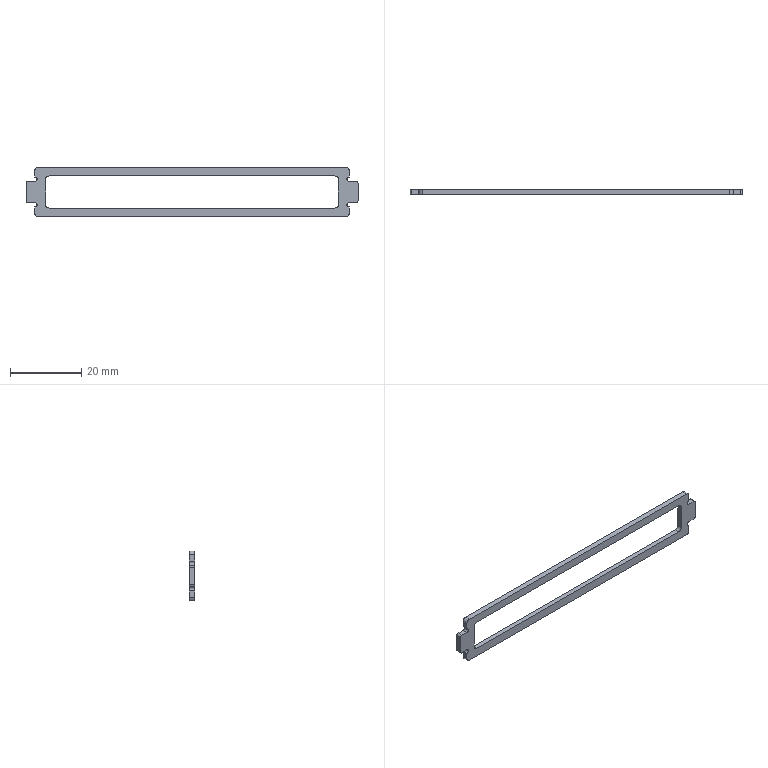Part | SolidWorks | features Fillet 2, Extrusion 1 | 1 solid | 34 faces | box 93.2 x 1.5 x 14 mm | volume 783.785 mm3 | plane 18 | cylinder 16 | commonest cylinder face diameters 2 x8 1 x4 1.2 x4
STEP:
#1=CARTESIAN_POINT('',(-44.1,1.5,-6.));
#2=VERTEX_POINT('',#1);
#3=CARTESIAN_POINT('',(-44.1,1.5,-4.2));
#4=VERTEX_POINT('',#3);
#5=CARTESIAN_POINT('',(-44.1,1.5,0.));
#6=DIRECTION('',(0.,0.,1.));
#7=VECTOR('',#6,1000.);
#8=LINE('',#5,#7);
#9=EDGE_CURVE('',#2,#4,#8,.T.);
#10=ORIENTED_EDGE('',*,*,#9,.F.);
#11=CARTESIAN_POINT('',(-44.1,0.,-6.));
#12=VERTEX_POINT('',#11);
#13=CARTESIAN_POINT('',(-44.1,0.,-6.));
#14=DIRECTION('',(0.,-1.,0.));
#15=VECTOR('',#14,1000.);
#16=LINE('',#13,#15);
#17=EDGE_CURVE('',#2,#12,#16,.T.);
#18=ORIENTED_EDGE('',*,*,#17,.T.);
#19=CARTESIAN_POINT('',(-44.1,0.,-4.2));
#20=VERTEX_POINT('',#19);
#21=CARTESIAN_POINT('',(-44.1,0.,0.));
#22=DIRECTION('',(0.,0.,1.));
#23=VECTOR('',#22,1000.);
#24=LINE('',#21,#23);
#25=EDGE_CURVE('',#12,#20,#24,.T.);
#26=ORIENTED_EDGE('',*,*,#25,.T.);
#27=CARTESIAN_POINT('',(-44.1,1.5,-4.2));
#28=DIRECTION('',(0.,-1.,0.));
#29=VECTOR('',#28,1000.);
#30=LINE('',#27,#29);
#31=EDGE_CURVE('',#4,#20,#30,.T.);
#32=ORIENTED_EDGE('',*,*,#31,.F.);
#33=EDGE_LOOP('',(#10,#18,#26,#32));
#34=FACE_OUTER_BOUND('',#33,.T.);
#35=CARTESIAN_POINT('',(-44.1,1.5,0.));
#36=DIRECTION('',(1.,0.,0.));
#37=DIRECTION('',(0.,0.,-1.));
#38=AXIS2_PLACEMENT_3D('',#35,#36,#37);
#39=PLANE('',#38);
#40=ADVANCED_FACE('',(#34),#39,.F.);
#41=CARTESIAN_POINT('',(-44.1,0.,-3.));
#42=VERTEX_POINT('',#41);
#43=CARTESIAN_POINT('',(-44.1,0.,-3.6));
#44=DIRECTION('',(0.,-1.,0.));
#45=DIRECTION('',(0.,0.,1.));
#46=AXIS2_PLACEMENT_3D('',#43,#44,#45);
#47=CIRCLE('',#46,0.6);
#48=EDGE_CURVE('',#20,#42,#47,.T.);
#49=ORIENTED_EDGE('',*,*,#48,.T.);
#50=CARTESIAN_POINT('',(-44.1,1.5,-3.));
#51=VERTEX_POINT('',#50);
#52=CARTESIAN_POINT('',(-44.1,1.5,-3.));
#53=DIRECTION('',(0.,-1.,0.));
#54=VECTOR('',#53,1000.);
#55=LINE('',#52,#54);
#56=EDGE_CURVE('',#51,#42,#55,.T.);
#57=ORIENTED_EDGE('',*,*,#56,.F.);
#58=CARTESIAN_POINT('',(-44.1,1.5,-3.6));
#59=DIRECTION('',(0.,-1.,0.));
#60=DIRECTION('',(0.,0.,1.));
#61=AXIS2_PLACEMENT_3D('',#58,#59,#60);
#62=CIRCLE('',#61,0.6);
#63=EDGE_CURVE('',#4,#51,#62,.T.);
#64=ORIENTED_EDGE('',*,*,#63,.F.);
#65=ORIENTED_EDGE('',*,*,#31,.T.);
#66=EDGE_LOOP('',(#49,#57,#64,#65));
#67=FACE_OUTER_BOUND('',#66,.T.);
#68=CARTESIAN_POINT('',(-44.1,1.5,-3.6));
#69=DIRECTION('',(0.,-1.,0.));
#70=DIRECTION('',(0.,0.,-1.));
#71=AXIS2_PLACEMENT_3D('',#68,#69,#70);
#72=CYLINDRICAL_SURFACE('',#71,0.6);
#73=ADVANCED_FACE('',(#67),#72,.F.);
#74=CARTESIAN_POINT('',(-46.1,0.,-3.));
#75=VERTEX_POINT('',#74);
#76=CARTESIAN_POINT('',(0.,0.,-3.));
#77=DIRECTION('',(-1.,0.,0.));
#78=VECTOR('',#77,1000.);
#79=LINE('',#76,#78);
#80=EDGE_CURVE('',#42,#75,#79,.T.);
#81=ORIENTED_EDGE('',*,*,#80,.T.);
#82=CARTESIAN_POINT('',(-46.1,1.5,-3.));
#83=VERTEX_POINT('',#82);
#84=CARTESIAN_POINT('',(-46.1,1.5,-3.));
#85=DIRECTION('',(0.,1.,0.));
#86=VECTOR('',#85,1000.);
#87=LINE('',#84,#86);
#88=EDGE_CURVE('',#75,#83,#87,.T.);
#89=ORIENTED_EDGE('',*,*,#88,.T.);
#90=CARTESIAN_POINT('',(0.,1.5,-3.));
#91=DIRECTION('',(-1.,0.,0.));
#92=VECTOR('',#91,1000.);
#93=LINE('',#90,#92);
#94=EDGE_CURVE('',#51,#83,#93,.T.);
#95=ORIENTED_EDGE('',*,*,#94,.F.);
#96=ORIENTED_EDGE('',*,*,#56,.T.);
#97=EDGE_LOOP('',(#81,#89,#95,#96));
#98=FACE_OUTER_BOUND('',#97,.T.);
#99=CARTESIAN_POINT('',(0.,1.5,-3.));
#100=DIRECTION('',(0.,0.,1.));
#101=DIRECTION('',(1.,0.,0.));
#102=AXIS2_PLACEMENT_3D('',#99,#100,#101);
#103=PLANE('',#102);
#104=ADVANCED_FACE('',(#98),#103,.F.);
#105=CARTESIAN_POINT('',(-46.6,0.,-2.5));
#106=VERTEX_POINT('',#105);
#107=CARTESIAN_POINT('',(-46.6,0.,2.5));
#108=VERTEX_POINT('',#107);
#109=CARTESIAN_POINT('',(-46.6,0.,0.));
#110=DIRECTION('',(0.,0.,1.));
#111=VECTOR('',#110,1000.);
#112=LINE('',#109,#111);
#113=EDGE_CURVE('',#106,#108,#112,.T.);
#114=ORIENTED_EDGE('',*,*,#113,.T.);
#115=CARTESIAN_POINT('',(-46.6,1.5,2.5));
#116=VERTEX_POINT('',#115);
#117=CARTESIAN_POINT('',(-46.6,1.5,2.5));
#118=DIRECTION('',(0.,1.,0.));
#119=VECTOR('',#118,1000.);
#120=LINE('',#117,#119);
#121=EDGE_CURVE('',#108,#116,#120,.T.);
#122=ORIENTED_EDGE('',*,*,#121,.T.);
#123=CARTESIAN_POINT('',(-46.6,1.5,-2.5));
#124=VERTEX_POINT('',#123);
#125=CARTESIAN_POINT('',(-46.6,1.5,0.));
#126=DIRECTION('',(0.,0.,1.));
#127=VECTOR('',#126,1000.);
#128=LINE('',#125,#127);
#129=EDGE_CURVE('',#124,#116,#128,.T.);
#130=ORIENTED_EDGE('',*,*,#129,.F.);
#131=CARTESIAN_POINT('',(-46.6,1.5,-2.5));
#132=DIRECTION('',(0.,-1.,0.));
#133=VECTOR('',#132,1000.);
#134=LINE('',#131,#133);
#135=EDGE_CURVE('',#124,#106,#134,.T.);
#136=ORIENTED_EDGE('',*,*,#135,.T.);
#137=EDGE_LOOP('',(#114,#122,#130,#136));
#138=FACE_OUTER_BOUND('',#137,.T.);
#139=CARTESIAN_POINT('',(-46.6,1.5,0.));
#140=DIRECTION('',(1.,0.,0.));
#141=DIRECTION('',(0.,0.,-1.));
#142=AXIS2_PLACEMENT_3D('',#139,#140,#141);
#143=PLANE('',#142);
#144=ADVANCED_FACE('',(#138),#143,.F.);
#145=CARTESIAN_POINT('',(-44.1,1.5,3.));
#146=VERTEX_POINT('',#145);
#147=CARTESIAN_POINT('',(-46.1,1.5,3.));
#148=VERTEX_POINT('',#147);
#149=CARTESIAN_POINT('',(0.,1.5,3.));
#150=DIRECTION('',(-1.,0.,0.));
#151=VECTOR('',#150,1000.);
#152=LINE('',#149,#151);
#153=EDGE_CURVE('',#146,#148,#152,.T.);
#154=ORIENTED_EDGE('',*,*,#153,.T.);
#155=CARTESIAN_POINT('',(-46.1,0.,3.));
#156=VERTEX_POINT('',#155);
#157=CARTESIAN_POINT('',(-46.1,0.,3.));
#158=DIRECTION('',(0.,-1.,0.));
#159=VECTOR('',#158,1000.);
#160=LINE('',#157,#159);
#161=EDGE_CURVE('',#148,#156,#160,.T.);
#162=ORIENTED_EDGE('',*,*,#161,.T.);
#163=CARTESIAN_POINT('',(-44.1,0.,3.));
#164=VERTEX_POINT('',#163);
#165=CARTESIAN_POINT('',(0.,0.,3.));
#166=DIRECTION('',(-1.,0.,0.));
#167=VECTOR('',#166,1000.);
#168=LINE('',#165,#167);
#169=EDGE_CURVE('',#164,#156,#168,.T.);
#170=ORIENTED_EDGE('',*,*,#169,.F.);
#171=CARTESIAN_POINT('',(-44.1,1.5,3.));
#172=DIRECTION('',(0.,-1.,0.));
#173=VECTOR('',#172,1000.);
#174=LINE('',#171,#173);
#175=EDGE_CURVE('',#146,#164,#174,.T.);
#176=ORIENTED_EDGE('',*,*,#175,.F.);
#177=EDGE_LOOP('',(#154,#162,#170,#176));
#178=FACE_OUTER_BOUND('',#177,.T.);
#179=CARTESIAN_POINT('',(0.,1.5,3.));
#180=DIRECTION('',(0.,0.,1.));
#181=DIRECTION('',(1.,0.,0.));
#182=AXIS2_PLACEMENT_3D('',#179,#180,#181);
#183=PLANE('',#182);
#184=ADVANCED_FACE('',(#178),#183,.T.);
#185=CARTESIAN_POINT('',(-44.1,0.,4.2));
#186=VERTEX_POINT('',#185);
#187=CARTESIAN_POINT('',(-44.1,0.,3.6));
#188=DIRECTION('',(0.,-1.,0.));
#189=DIRECTION('',(0.,0.,1.));
#190=AXIS2_PLACEMENT_3D('',#187,#188,#189);
#191=CIRCLE('',#190,0.6);
#192=EDGE_CURVE('',#164,#186,#191,.T.);
#193=ORIENTED_EDGE('',*,*,#192,.T.);
#194=CARTESIAN_POINT('',(-44.1,1.5,4.2));
#195=VERTEX_POINT('',#194);
#196=CARTESIAN_POINT('',(-44.1,1.5,4.2));
#197=DIRECTION('',(0.,-1.,0.));
#198=VECTOR('',#197,1000.);
#199=LINE('',#196,#198);
#200=EDGE_CURVE('',#195,#186,#199,.T.);
#201=ORIENTED_EDGE('',*,*,#200,.F.);
#202=CARTESIAN_POINT('',(-44.1,1.5,3.6));
#203=DIRECTION('',(0.,-1.,0.));
#204=DIRECTION('',(0.,0.,1.));
#205=AXIS2_PLACEMENT_3D('',#202,#203,#204);
#206=CIRCLE('',#205,0.6);
#207=EDGE_CURVE('',#146,#195,#206,.T.);
#208=ORIENTED_EDGE('',*,*,#207,.F.);
#209=ORIENTED_EDGE('',*,*,#175,.T.);
#210=EDGE_LOOP('',(#193,#201,#208,#209));
#211=FACE_OUTER_BOUND('',#210,.T.);
#212=CARTESIAN_POINT('',(-44.1,1.5,3.6));
#213=DIRECTION('',(0.,-1.,0.));
#214=DIRECTION('',(0.,0.,-1.));
#215=AXIS2_PLACEMENT_3D('',#212,#213,#214);
#216=CYLINDRICAL_SURFACE('',#215,0.6);
#217=ADVANCED_FACE('',(#211),#216,.F.);
#218=CARTESIAN_POINT('',(-44.1,0.,6.));
#219=VERTEX_POINT('',#218);
#220=CARTESIAN_POINT('',(-44.1,0.,0.));
#221=DIRECTION('',(0.,0.,1.));
#222=VECTOR('',#221,1000.);
#223=LINE('',#220,#222);
#224=EDGE_CURVE('',#186,#219,#223,.T.);
#225=ORIENTED_EDGE('',*,*,#224,.T.);
#226=CARTESIAN_POINT('',(-44.1,1.5,6.));
#227=VERTEX_POINT('',#226);
#228=CARTESIAN_POINT('',(-44.1,1.5,6.));
#229=DIRECTION('',(0.,1.,0.));
#230=VECTOR('',#229,1000.);
#231=LINE('',#228,#230);
#232=EDGE_CURVE('',#219,#227,#231,.T.);
#233=ORIENTED_EDGE('',*,*,#232,.T.);
#234=CARTESIAN_POINT('',(-44.1,1.5,0.));
#235=DIRECTION('',(0.,0.,1.));
#236=VECTOR('',#235,1000.);
#237=LINE('',#234,#236);
#238=EDGE_CURVE('',#195,#227,#237,.T.);
#239=ORIENTED_EDGE('',*,*,#238,.F.);
#240=ORIENTED_EDGE('',*,*,#200,.T.);
#241=EDGE_LOOP('',(#225,#233,#239,#240));
#242=FACE_OUTER_BOUND('',#241,.T.);
#243=CARTESIAN_POINT('',(-44.1,1.5,0.));
#244=DIRECTION('',(1.,0.,0.));
#245=DIRECTION('',(0.,0.,-1.));
#246=AXIS2_PLACEMENT_3D('',#243,#244,#245);
#247=PLANE('',#246);
#248=ADVANCED_FACE('',(#242),#247,.F.);
#249=CARTESIAN_POINT('',(-43.1,1.5,7.));
#250=VERTEX_POINT('',#249);
#251=CARTESIAN_POINT('',(43.1,1.5,7.));
#252=VERTEX_POINT('',#251);
#253=CARTESIAN_POINT('',(0.,1.5,7.));
#254=DIRECTION('',(1.,0.,0.));
#255=VECTOR('',#254,1000.);
#256=LINE('',#253,#255);
#257=EDGE_CURVE('',#250,#252,#256,.T.);
#258=ORIENTED_EDGE('',*,*,#257,.F.);
#259=CARTESIAN_POINT('',(-43.1,0.,7.));
#260=VERTEX_POINT('',#259);
#261=CARTESIAN_POINT('',(-43.1,1.5,7.));
#262=DIRECTION('',(0.,-1.,0.));
#263=VECTOR('',#262,1000.);
#264=LINE('',#261,#263);
#265=EDGE_CURVE('',#250,#260,#264,.T.);
#266=ORIENTED_EDGE('',*,*,#265,.T.);
#267=CARTESIAN_POINT('',(43.1,0.,7.));
#268=VERTEX_POINT('',#267);
#269=CARTESIAN_POINT('',(0.,0.,7.));
#270=DIRECTION('',(1.,0.,0.));
#271=VECTOR('',#270,1000.);
#272=LINE('',#269,#271);
#273=EDGE_CURVE('',#260,#268,#272,.T.);
#274=ORIENTED_EDGE('',*,*,#273,.T.);
#275=CARTESIAN_POINT('',(43.1,1.5,7.));
#276=DIRECTION('',(0.,1.,0.));
#277=VECTOR('',#276,1000.);
#278=LINE('',#275,#277);
#279=EDGE_CURVE('',#268,#252,#278,.T.);
#280=ORIENTED_EDGE('',*,*,#279,.T.);
#281=EDGE_LOOP('',(#258,#266,#274,#280));
#282=FACE_OUTER_BOUND('',#281,.T.);
#283=CARTESIAN_POINT('',(0.,1.5,7.));
#284=DIRECTION('',(0.,0.,-1.));
#285=DIRECTION('',(-1.,0.,0.));
#286=AXIS2_PLACEMENT_3D('',#283,#284,#285);
#287=PLANE('',#286);
#288=ADVANCED_FACE('',(#282),#287,.F.);
#289=CARTESIAN_POINT('',(44.1,1.5,4.2));
#290=VERTEX_POINT('',#289);
#291=CARTESIAN_POINT('',(44.1,1.5,6.));
#292=VERTEX_POINT('',#291);
#293=CARTESIAN_POINT('',(44.1,1.5,0.));
#294=DIRECTION('',(0.,0.,1.));
#295=VECTOR('',#294,1000.);
#296=LINE('',#293,#295);
#297=EDGE_CURVE('',#290,#292,#296,.T.);
#298=ORIENTED_EDGE('',*,*,#297,.T.);
#299=CARTESIAN_POINT('',(44.1,0.,6.));
#300=VERTEX_POINT('',#299);
#301=CARTESIAN_POINT('',(44.1,0.,6.));
#302=DIRECTION('',(0.,-1.,0.));
#303=VECTOR('',#302,1000.);
#304=LINE('',#301,#303);
#305=EDGE_CURVE('',#292,#300,#304,.T.);
#306=ORIENTED_EDGE('',*,*,#305,.T.);
#307=CARTESIAN_POINT('',(44.1,0.,4.2));
#308=VERTEX_POINT('',#307);
#309=CARTESIAN_POINT('',(44.1,0.,0.));
#310=DIRECTION('',(0.,0.,1.));
#311=VECTOR('',#310,1000.);
#312=LINE('',#309,#311);
#313=EDGE_CURVE('',#308,#300,#312,.T.);
#314=ORIENTED_EDGE('',*,*,#313,.F.);
#315=CARTESIAN_POINT('',(44.1,1.5,4.2));
#316=DIRECTION('',(0.,-1.,0.));
#317=VECTOR('',#316,1000.);
#318=LINE('',#315,#317);
#319=EDGE_CURVE('',#290,#308,#318,.T.);
#320=ORIENTED_EDGE('',*,*,#319,.F.);
#321=EDGE_LOOP('',(#298,#306,#314,#320));
#322=FACE_OUTER_BOUND('',#321,.T.);
#323=CARTESIAN_POINT('',(44.1,1.5,0.));
#324=DIRECTION('',(1.,0.,0.));
#325=DIRECTION('',(0.,0.,-1.));
#326=AXIS2_PLACEMENT_3D('',#323,#324,#325);
#327=PLANE('',#326);
#328=ADVANCED_FACE('',(#322),#327,.T.);
#329=CARTESIAN_POINT('',(44.1,0.,3.));
#330=VERTEX_POINT('',#329);
#331=CARTESIAN_POINT('',(44.1,0.,3.6));
#332=DIRECTION('',(0.,1.,0.));
#333=DIRECTION('',(0.,0.,1.));
#334=AXIS2_PLACEMENT_3D('',#331,#332,#333);
#335=CIRCLE('',#334,0.6);
#336=EDGE_CURVE('',#330,#308,#335,.T.);
#337=ORIENTED_EDGE('',*,*,#336,.F.);
#338=CARTESIAN_POINT('',(44.1,1.5,3.));
#339=VERTEX_POINT('',#338);
#340=CARTESIAN_POINT('',(44.1,1.5,3.));
#341=DIRECTION('',(0.,-1.,0.));
#342=VECTOR('',#341,1000.);
#343=LINE('',#340,#342);
#344=EDGE_CURVE('',#339,#330,#343,.T.);
#345=ORIENTED_EDGE('',*,*,#344,.F.);
#346=CARTESIAN_POINT('',(44.1,1.5,3.6));
#347=DIRECTION('',(0.,1.,0.));
#348=DIRECTION('',(0.,0.,1.));
#349=AXIS2_PLACEMENT_3D('',#346,#347,#348);
#350=CIRCLE('',#349,0.6);
#351=EDGE_CURVE('',#339,#290,#350,.T.);
#352=ORIENTED_EDGE('',*,*,#351,.T.);
#353=ORIENTED_EDGE('',*,*,#319,.T.);
#354=EDGE_LOOP('',(#337,#345,#352,#353));
#355=FACE_OUTER_BOUND('',#354,.T.);
#356=CARTESIAN_POINT('',(44.1,1.5,3.6));
#357=DIRECTION('',(0.,-1.,0.));
#358=DIRECTION('',(0.,0.,-1.));
#359=AXIS2_PLACEMENT_3D('',#356,#357,#358);
#360=CYLINDRICAL_SURFACE('',#359,0.6);
#361=ADVANCED_FACE('',(#355),#360,.F.);
#362=CARTESIAN_POINT('',(46.1,0.,3.));
#363=VERTEX_POINT('',#362);
#364=CARTESIAN_POINT('',(0.,0.,3.));
#365=DIRECTION('',(1.,0.,0.));
#366=VECTOR('',#365,1000.);
#367=LINE('',#364,#366);
#368=EDGE_CURVE('',#330,#363,#367,.T.);
#369=ORIENTED_EDGE('',*,*,#368,.T.);
#370=CARTESIAN_POINT('',(46.1,1.5,3.));
#371=VERTEX_POINT('',#370);
#372=CARTESIAN_POINT('',(46.1,1.5,3.));
#373=DIRECTION('',(0.,1.,0.));
#374=VECTOR('',#373,1000.);
#375=LINE('',#372,#374);
#376=EDGE_CURVE('',#363,#371,#375,.T.);
#377=ORIENTED_EDGE('',*,*,#376,.T.);
#378=CARTESIAN_POINT('',(0.,1.5,3.));
#379=DIRECTION('',(1.,0.,0.));
#380=VECTOR('',#379,1000.);
#381=LINE('',#378,#380);
#382=EDGE_CURVE('',#339,#371,#381,.T.);
#383=ORIENTED_EDGE('',*,*,#382,.F.);
#384=ORIENTED_EDGE('',*,*,#344,.T.);
#385=EDGE_LOOP('',(#369,#377,#383,#384));
#386=FACE_OUTER_BOUND('',#385,.T.);
#387=CARTESIAN_POINT('',(0.,1.5,3.));
#388=DIRECTION('',(0.,0.,-1.));
#389=DIRECTION('',(-1.,0.,0.));
#390=AXIS2_PLACEMENT_3D('',#387,#388,#389);
#391=PLANE('',#390);
#392=ADVANCED_FACE('',(#386),#391,.F.);
#393=CARTESIAN_POINT('',(46.6,1.5,-2.5));
#394=VERTEX_POINT('',#393);
#395=CARTESIAN_POINT('',(46.6,1.5,2.5));
#396=VERTEX_POINT('',#395);
#397=CARTESIAN_POINT('',(46.6,1.5,0.));
#398=DIRECTION('',(0.,0.,1.));
#399=VECTOR('',#398,1000.);
#400=LINE('',#397,#399);
#401=EDGE_CURVE('',#394,#396,#400,.T.);
#402=ORIENTED_EDGE('',*,*,#401,.T.);
#403=CARTESIAN_POINT('',(46.6,0.,2.5));
#404=VERTEX_POINT('',#403);
#405=CARTESIAN_POINT('',(46.6,0.,2.5));
#406=DIRECTION('',(0.,-1.,0.));
#407=VECTOR('',#406,1000.);
#408=LINE('',#405,#407);
#409=EDGE_CURVE('',#396,#404,#408,.T.);
#410=ORIENTED_EDGE('',*,*,#409,.T.);
#411=CARTESIAN_POINT('',(46.6,0.,-2.5));
#412=VERTEX_POINT('',#411);
#413=CARTESIAN_POINT('',(46.6,0.,0.));
#414=DIRECTION('',(0.,0.,1.));
#415=VECTOR('',#414,1000.);
#416=LINE('',#413,#415);
#417=EDGE_CURVE('',#412,#404,#416,.T.);
#418=ORIENTED_EDGE('',*,*,#417,.F.);
#419=CARTESIAN_POINT('',(46.6,1.5,-2.5));
#420=DIRECTION('',(0.,1.,0.));
#421=VECTOR('',#420,1000.);
#422=LINE('',#419,#421);
#423=EDGE_CURVE('',#412,#394,#422,.T.);
#424=ORIENTED_EDGE('',*,*,#423,.T.);
#425=EDGE_LOOP('',(#402,#410,#418,#424));
#426=FACE_OUTER_BOUND('',#425,.T.);
#427=CARTESIAN_POINT('',(46.6,1.5,0.));
#428=DIRECTION('',(1.,0.,0.));
#429=DIRECTION('',(0.,0.,-1.));
#430=AXIS2_PLACEMENT_3D('',#427,#428,#429);
#431=PLANE('',#430);
#432=ADVANCED_FACE('',(#426),#431,.T.);
#433=CARTESIAN_POINT('',(44.1,1.5,-3.));
#434=VERTEX_POINT('',#433);
#435=CARTESIAN_POINT('',(46.1,1.5,-3.));
#436=VERTEX_POINT('',#435);
#437=CARTESIAN_POINT('',(0.,1.5,-3.));
#438=DIRECTION('',(1.,0.,0.));
#439=VECTOR('',#438,1000.);
#440=LINE('',#437,#439);
#441=EDGE_CURVE('',#434,#436,#440,.T.);
#442=ORIENTED_EDGE('',*,*,#441,.T.);
#443=CARTESIAN_POINT('',(46.1,0.,-3.));
#444=VERTEX_POINT('',#443);
#445=CARTESIAN_POINT('',(46.1,1.5,-3.));
#446=DIRECTION('',(0.,-1.,0.));
#447=VECTOR('',#446,1000.);
#448=LINE('',#445,#447);
#449=EDGE_CURVE('',#436,#444,#448,.T.);
#450=ORIENTED_EDGE('',*,*,#449,.T.);
#451=CARTESIAN_POINT('',(44.1,0.,-3.));
#452=VERTEX_POINT('',#451);
#453=CARTESIAN_POINT('',(0.,0.,-3.));
#454=DIRECTION('',(1.,0.,0.));
#455=VECTOR('',#454,1000.);
#456=LINE('',#453,#455);
#457=EDGE_CURVE('',#452,#444,#456,.T.);
#458=ORIENTED_EDGE('',*,*,#457,.F.);
#459=CARTESIAN_POINT('',(44.1,1.5,-3.));
#460=DIRECTION('',(0.,-1.,0.));
#461=VECTOR('',#460,1000.);
#462=LINE('',#459,#461);
#463=EDGE_CURVE('',#434,#452,#462,.T.);
#464=ORIENTED_EDGE('',*,*,#463,.F.);
#465=EDGE_LOOP('',(#442,#450,#458,#464));
#466=FACE_OUTER_BOUND('',#465,.T.);
#467=CARTESIAN_POINT('',(0.,1.5,-3.));
#468=DIRECTION('',(0.,0.,-1.));
#469=DIRECTION('',(-1.,0.,0.));
#470=AXIS2_PLACEMENT_3D('',#467,#468,#469);
#471=PLANE('',#470);
#472=ADVANCED_FACE('',(#466),#471,.T.);
#473=CARTESIAN_POINT('',(44.1,0.,-4.2));
#474=VERTEX_POINT('',#473);
#475=CARTESIAN_POINT('',(44.1,0.,-3.6));
#476=DIRECTION('',(0.,1.,0.));
#477=DIRECTION('',(0.,0.,1.));
#478=AXIS2_PLACEMENT_3D('',#475,#476,#477);
#479=CIRCLE('',#478,0.6);
#480=EDGE_CURVE('',#474,#452,#479,.T.);
#481=ORIENTED_EDGE('',*,*,#480,.F.);
#482=CARTESIAN_POINT('',(44.1,1.5,-4.2));
#483=VERTEX_POINT('',#482);
#484=CARTESIAN_POINT('',(44.1,1.5,-4.2));
#485=DIRECTION('',(0.,-1.,0.));
#486=VECTOR('',#485,1000.);
#487=LINE('',#484,#486);
#488=EDGE_CURVE('',#483,#474,#487,.T.);
#489=ORIENTED_EDGE('',*,*,#488,.F.);
#490=CARTESIAN_POINT('',(44.1,1.5,-3.6));
#491=DIRECTION('',(0.,1.,0.));
#492=DIRECTION('',(0.,0.,1.));
#493=AXIS2_PLACEMENT_3D('',#490,#491,#492);
#494=CIRCLE('',#493,0.6);
#495=EDGE_CURVE('',#483,#434,#494,.T.);
#496=ORIENTED_EDGE('',*,*,#495,.T.);
#497=ORIENTED_EDGE('',*,*,#463,.T.);
#498=EDGE_LOOP('',(#481,#489,#496,#497));
#499=FACE_OUTER_BOUND('',#498,.T.);
#500=CARTESIAN_POINT('',(44.1,1.5,-3.6));
#501=DIRECTION('',(0.,-1.,0.));
#502=DIRECTION('',(0.,0.,-1.));
#503=AXIS2_PLACEMENT_3D('',#500,#501,#502);
#504=CYLINDRICAL_SURFACE('',#503,0.6);
#505=ADVANCED_FACE('',(#499),#504,.F.);
#506=CARTESIAN_POINT('',(44.1,0.,-6.));
#507=VERTEX_POINT('',#506);
#508=CARTESIAN_POINT('',(44.1,0.,0.));
#509=DIRECTION('',(0.,0.,1.));
#510=VECTOR('',#509,1000.);
#511=LINE('',#508,#510);
#512=EDGE_CURVE('',#507,#474,#511,.T.);
#513=ORIENTED_EDGE('',*,*,#512,.F.);
#514=CARTESIAN_POINT('',(44.1,1.5,-6.));
#515=VERTEX_POINT('',#514);
#516=CARTESIAN_POINT('',(44.1,1.5,-6.));
#517=DIRECTION('',(0.,1.,0.));
#518=VECTOR('',#517,1000.);
#519=LINE('',#516,#518);
#520=EDGE_CURVE('',#507,#515,#519,.T.);
#521=ORIENTED_EDGE('',*,*,#520,.T.);
#522=CARTESIAN_POINT('',(44.1,1.5,0.));
#523=DIRECTION('',(0.,0.,1.));
#524=VECTOR('',#523,1000.);
#525=LINE('',#522,#524);
#526=EDGE_CURVE('',#515,#483,#525,.T.);
#527=ORIENTED_EDGE('',*,*,#526,.T.);
#528=ORIENTED_EDGE('',*,*,#488,.T.);
#529=EDGE_LOOP('',(#513,#521,#527,#528));
#530=FACE_OUTER_BOUND('',#529,.T.);
#531=CARTESIAN_POINT('',(44.1,1.5,0.));
#532=DIRECTION('',(1.,0.,0.));
#533=DIRECTION('',(0.,0.,-1.));
#534=AXIS2_PLACEMENT_3D('',#531,#532,#533);
#535=PLANE('',#534);
#536=ADVANCED_FACE('',(#530),#535,.T.);
#537=CARTESIAN_POINT('',(-40.1,0.,-4.5));
#538=VERTEX_POINT('',#537);
#539=CARTESIAN_POINT('',(40.1,0.,-4.5));
#540=VERTEX_POINT('',#539);
#541=CARTESIAN_POINT('',(0.,0.,-4.5));
#542=DIRECTION('',(1.,0.,0.));
#543=VECTOR('',#542,1000.);
#544=LINE('',#541,#543);
#545=EDGE_CURVE('',#538,#540,#544,.T.);
#546=ORIENTED_EDGE('',*,*,#545,.T.);
#547=CARTESIAN_POINT('',(40.1,1.5,-4.5));
#548=VERTEX_POINT('',#547);
#549=CARTESIAN_POINT('',(40.1,1.5,-4.5));
#550=DIRECTION('',(0.,1.,0.));
#551=VECTOR('',#550,1000.);
#552=LINE('',#549,#551);
#553=EDGE_CURVE('',#540,#548,#552,.T.);
#554=ORIENTED_EDGE('',*,*,#553,.T.);
#555=CARTESIAN_POINT('',(-40.1,1.5,-4.5));
#556=VERTEX_POINT('',#555);
#557=CARTESIAN_POINT('',(0.,1.5,-4.5));
#558=DIRECTION('',(1.,0.,0.));
#559=VECTOR('',#558,1000.);
#560=LINE('',#557,#559);
#561=EDGE_CURVE('',#556,#548,#560,.T.);
#562=ORIENTED_EDGE('',*,*,#561,.F.);
#563=CARTESIAN_POINT('',(-40.1,1.5,-4.5));
#564=DIRECTION('',(0.,-1.,0.));
#565=VECTOR('',#564,1000.);
#566=LINE('',#563,#565);
#567=EDGE_CURVE('',#556,#538,#566,.T.);
#568=ORIENTED_EDGE('',*,*,#567,.T.);
#569=EDGE_LOOP('',(#546,#554,#562,#568));
#570=FACE_OUTER_BOUND('',#569,.T.);
#571=CARTESIAN_POINT('',(0.,1.5,-4.5));
#572=DIRECTION('',(0.,0.,-1.));
#573=DIRECTION('',(-1.,0.,0.));
#574=AXIS2_PLACEMENT_3D('',#571,#572,#573);
#575=PLANE('',#574);
#576=ADVANCED_FACE('',(#570),#575,.F.);
#577=CARTESIAN_POINT('',(41.1,0.,-3.5));
#578=VERTEX_POINT('',#577);
#579=CARTESIAN_POINT('',(41.1,0.,3.5));
#580=VERTEX_POINT('',#579);
#581=CARTESIAN_POINT('',(41.1,0.,0.));
#582=DIRECTION('',(0.,0.,1.));
#583=VECTOR('',#582,1000.);
#584=LINE('',#581,#583);
#585=EDGE_CURVE('',#578,#580,#584,.T.);
#586=ORIENTED_EDGE('',*,*,#585,.T.);
#587=CARTESIAN_POINT('',(41.1,1.5,3.5));
#588=VERTEX_POINT('',#587);
#589=CARTESIAN_POINT('',(41.1,1.5,3.5));
#590=DIRECTION('',(0.,1.,0.));
#591=VECTOR('',#590,1000.);
#592=LINE('',#589,#591);
#593=EDGE_CURVE('',#580,#588,#592,.T.);
#594=ORIENTED_EDGE('',*,*,#593,.T.);
#595=CARTESIAN_POINT('',(41.1,1.5,-3.5));
#596=VERTEX_POINT('',#595);
#597=CARTESIAN_POINT('',(41.1,1.5,0.));
#598=DIRECTION('',(0.,0.,1.));
#599=VECTOR('',#598,1000.);
#600=LINE('',#597,#599);
#601=EDGE_CURVE('',#596,#588,#600,.T.);
#602=ORIENTED_EDGE('',*,*,#601,.F.);
#603=CARTESIAN_POINT('',(41.1,0.,-3.5));
#604=DIRECTION('',(0.,-1.,0.));
#605=VECTOR('',#604,1000.);
#606=LINE('',#603,#605);
#607=EDGE_CURVE('',#596,#578,#606,.T.);
#608=ORIENTED_EDGE('',*,*,#607,.T.);
#609=EDGE_LOOP('',(#586,#594,#602,#608));
#610=FACE_OUTER_BOUND('',#609,.T.);
#611=CARTESIAN_POINT('',(41.1,1.5,0.));
#612=DIRECTION('',(1.,0.,0.));
#613=DIRECTION('',(0.,0.,-1.));
#614=AXIS2_PLACEMENT_3D('',#611,#612,#613);
#615=PLANE('',#614);
#616=ADVANCED_FACE('',(#610),#615,.F.);
#617=CARTESIAN_POINT('',(-40.1,0.,4.5));
#618=VERTEX_POINT('',#617);
#619=CARTESIAN_POINT('',(40.1,0.,4.5));
#620=VERTEX_POINT('',#619);
#621=CARTESIAN_POINT('',(0.,0.,4.5));
#622=DIRECTION('',(1.,0.,0.));
#623=VECTOR('',#622,1000.);
#624=LINE('',#621,#623);
#625=EDGE_CURVE('',#618,#620,#624,.T.);
#626=ORIENTED_EDGE('',*,*,#625,.F.);
#627=CARTESIAN_POINT('',(-40.1,1.5,4.5));
#628=VERTEX_POINT('',#627);
#629=CARTESIAN_POINT('',(-40.1,1.5,4.5));
#630=DIRECTION('',(0.,1.,0.));
#631=VECTOR('',#630,1000.);
#632=LINE('',#629,#631);
#633=EDGE_CURVE('',#618,#628,#632,.T.);
#634=ORIENTED_EDGE('',*,*,#633,.T.);
#635=CARTESIAN_POINT('',(40.1,1.5,4.5));
#636=VERTEX_POINT('',#635);
#637=CARTESIAN_POINT('',(0.,1.5,4.5));
#638=DIRECTION('',(1.,0.,0.));
#639=VECTOR('',#638,1000.);
#640=LINE('',#637,#639);
#641=EDGE_CURVE('',#628,#636,#640,.T.);
#642=ORIENTED_EDGE('',*,*,#641,.T.);
#643=CARTESIAN_POINT('',(40.1,1.5,4.5));
#644=DIRECTION('',(0.,-1.,0.));
#645=VECTOR('',#644,1000.);
#646=LINE('',#643,#645);
#647=EDGE_CURVE('',#636,#620,#646,.T.);
#648=ORIENTED_EDGE('',*,*,#647,.T.);
#649=EDGE_LOOP('',(#626,#634,#642,#648));
#650=FACE_OUTER_BOUND('',#649,.T.);
#651=CARTESIAN_POINT('',(0.,1.5,4.5));
#652=DIRECTION('',(0.,0.,-1.));
#653=DIRECTION('',(-1.,0.,0.));
#654=AXIS2_PLACEMENT_3D('',#651,#652,#653);
#655=PLANE('',#654);
#656=ADVANCED_FACE('',(#650),#655,.T.);
#657=CARTESIAN_POINT('',(-41.1,1.5,-3.5));
#658=VERTEX_POINT('',#657);
#659=CARTESIAN_POINT('',(-41.1,1.5,3.5));
#660=VERTEX_POINT('',#659);
#661=CARTESIAN_POINT('',(-41.1,1.5,0.));
#662=DIRECTION('',(0.,0.,1.));
#663=VECTOR('',#662,1000.);
#664=LINE('',#661,#663);
#665=EDGE_CURVE('',#658,#660,#664,.T.);
#666=ORIENTED_EDGE('',*,*,#665,.T.);
#667=CARTESIAN_POINT('',(-41.1,0.,3.5));
#668=VERTEX_POINT('',#667);
#669=CARTESIAN_POINT('',(-41.1,0.,3.5));
#670=DIRECTION('',(0.,-1.,0.));
#671=VECTOR('',#670,1000.);
#672=LINE('',#669,#671);
#673=EDGE_CURVE('',#660,#668,#672,.T.);
#674=ORIENTED_EDGE('',*,*,#673,.T.);
#675=CARTESIAN_POINT('',(-41.1,0.,-3.5));
#676=VERTEX_POINT('',#675);
#677=CARTESIAN_POINT('',(-41.1,0.,0.));
#678=DIRECTION('',(0.,0.,1.));
#679=VECTOR('',#678,1000.);
#680=LINE('',#677,#679);
#681=EDGE_CURVE('',#676,#668,#680,.T.);
#682=ORIENTED_EDGE('',*,*,#681,.F.);
#683=CARTESIAN_POINT('',(-41.1,1.5,-3.5));
#684=DIRECTION('',(0.,1.,0.));
#685=VECTOR('',#684,1000.);
#686=LINE('',#683,#685);
#687=EDGE_CURVE('',#676,#658,#686,.T.);
#688=ORIENTED_EDGE('',*,*,#687,.T.);
#689=EDGE_LOOP('',(#666,#674,#682,#688));
#690=FACE_OUTER_BOUND('',#689,.T.);
#691=CARTESIAN_POINT('',(-41.1,1.5,0.));
#692=DIRECTION('',(1.,0.,0.));
#693=DIRECTION('',(0.,0.,-1.));
#694=AXIS2_PLACEMENT_3D('',#691,#692,#693);
#695=PLANE('',#694);
#696=ADVANCED_FACE('',(#690),#695,.T.);
#697=CARTESIAN_POINT('',(-43.1,0.,-7.));
#698=VERTEX_POINT('',#697);
#699=CARTESIAN_POINT('',(43.1,0.,-7.));
#700=VERTEX_POINT('',#699);
#701=CARTESIAN_POINT('',(0.,0.,-7.));
#702=DIRECTION('',(1.,0.,0.));
#703=VECTOR('',#702,1000.);
#704=LINE('',#701,#703);
#705=EDGE_CURVE('',#698,#700,#704,.T.);
#706=ORIENTED_EDGE('',*,*,#705,.F.);
#707=CARTESIAN_POINT('',(-43.1,1.5,-7.));
#708=VERTEX_POINT('',#707);
#709=CARTESIAN_POINT('',(-43.1,1.5,-7.));
#710=DIRECTION('',(0.,1.,0.));
#711=VECTOR('',#710,1000.);
#712=LINE('',#709,#711);
#713=EDGE_CURVE('',#698,#708,#712,.T.);
#714=ORIENTED_EDGE('',*,*,#713,.T.);
#715=CARTESIAN_POINT('',(43.1,1.5,-7.));
#716=VERTEX_POINT('',#715);
#717=CARTESIAN_POINT('',(0.,1.5,-7.));
#718=DIRECTION('',(1.,0.,0.));
#719=VECTOR('',#718,1000.);
#720=LINE('',#717,#719);
#721=EDGE_CURVE('',#708,#716,#720,.T.);
#722=ORIENTED_EDGE('',*,*,#721,.T.);
#723=CARTESIAN_POINT('',(43.1,1.5,-7.));
#724=DIRECTION('',(0.,-1.,0.));
#725=VECTOR('',#724,1000.);
#726=LINE('',#723,#725);
#727=EDGE_CURVE('',#716,#700,#726,.T.);
#728=ORIENTED_EDGE('',*,*,#727,.T.);
#729=EDGE_LOOP('',(#706,#714,#722,#728));
#730=FACE_OUTER_BOUND('',#729,.T.);
#731=CARTESIAN_POINT('',(0.,1.5,-7.));
#732=DIRECTION('',(0.,0.,-1.));
#733=DIRECTION('',(-1.,0.,0.));
#734=AXIS2_PLACEMENT_3D('',#731,#732,#733);
#735=PLANE('',#734);
#736=ADVANCED_FACE('',(#730),#735,.T.);
#737=ORIENTED_EDGE('',*,*,#665,.F.);
#738=CARTESIAN_POINT('',(-40.1,1.5,-3.5));
#739=DIRECTION('',(0.,-1.,0.));
#740=DIRECTION('',(0.,0.,1.));
#741=AXIS2_PLACEMENT_3D('',#738,#739,#740);
#742=CIRCLE('',#741,1.);
#743=EDGE_CURVE('',#658,#556,#742,.T.);
#744=ORIENTED_EDGE('',*,*,#743,.T.);
#745=ORIENTED_EDGE('',*,*,#561,.T.);
#746=CARTESIAN_POINT('',(40.1,1.5,-3.5));
#747=DIRECTION('',(0.,-1.,0.));
#748=DIRECTION('',(0.,0.,1.));
#749=AXIS2_PLACEMENT_3D('',#746,#747,#748);
#750=CIRCLE('',#749,1.);
#751=EDGE_CURVE('',#548,#596,#750,.T.);
#752=ORIENTED_EDGE('',*,*,#751,.T.);
#753=ORIENTED_EDGE('',*,*,#601,.T.);
#754=CARTESIAN_POINT('',(40.1,1.5,3.5));
#755=DIRECTION('',(0.,-1.,0.));
#756=DIRECTION('',(0.,0.,1.));
#757=AXIS2_PLACEMENT_3D('',#754,#755,#756);
#758=CIRCLE('',#757,1.);
#759=EDGE_CURVE('',#588,#636,#758,.T.);
#760=ORIENTED_EDGE('',*,*,#759,.T.);
#761=ORIENTED_EDGE('',*,*,#641,.F.);
#762=CARTESIAN_POINT('',(-40.1,1.5,3.5));
#763=DIRECTION('',(0.,-1.,0.));
#764=DIRECTION('',(0.,0.,1.));
#765=AXIS2_PLACEMENT_3D('',#762,#763,#764);
#766=CIRCLE('',#765,1.);
#767=EDGE_CURVE('',#628,#660,#766,.T.);
#768=ORIENTED_EDGE('',*,*,#767,.T.);
#769=EDGE_LOOP('',(#737,#744,#745,#752,#753,#760,#761,#768));
#770=FACE_BOUND('',#769,.T.);
#771=ORIENTED_EDGE('',*,*,#721,.F.);
#772=CARTESIAN_POINT('',(-43.1,1.5,-6.));
#773=DIRECTION('',(0.,1.,0.));
#774=DIRECTION('',(0.,0.,1.));
#775=AXIS2_PLACEMENT_3D('',#772,#773,#774);
#776=CIRCLE('',#775,1.);
#777=EDGE_CURVE('',#708,#2,#776,.T.);
#778=ORIENTED_EDGE('',*,*,#777,.T.);
#779=ORIENTED_EDGE('',*,*,#9,.T.);
#780=ORIENTED_EDGE('',*,*,#63,.T.);
#781=ORIENTED_EDGE('',*,*,#94,.T.);
#782=CARTESIAN_POINT('',(-46.1,1.5,-2.5));
#783=DIRECTION('',(0.,1.,0.));
#784=DIRECTION('',(0.,0.,1.));
#785=AXIS2_PLACEMENT_3D('',#782,#783,#784);
#786=CIRCLE('',#785,0.5);
#787=EDGE_CURVE('',#83,#124,#786,.T.);
#788=ORIENTED_EDGE('',*,*,#787,.T.);
#789=ORIENTED_EDGE('',*,*,#129,.T.);
#790=CARTESIAN_POINT('',(-46.1,1.5,2.5));
#791=DIRECTION('',(0.,1.,0.));
#792=DIRECTION('',(0.,0.,1.));
#793=AXIS2_PLACEMENT_3D('',#790,#791,#792);
#794=CIRCLE('',#793,0.5);
#795=EDGE_CURVE('',#116,#148,#794,.T.);
#796=ORIENTED_EDGE('',*,*,#795,.T.);
#797=ORIENTED_EDGE('',*,*,#153,.F.);
#798=ORIENTED_EDGE('',*,*,#207,.T.);
#799=ORIENTED_EDGE('',*,*,#238,.T.);
#800=CARTESIAN_POINT('',(-43.1,1.5,6.));
#801=DIRECTION('',(0.,1.,0.));
#802=DIRECTION('',(0.,0.,1.));
#803=AXIS2_PLACEMENT_3D('',#800,#801,#802);
#804=CIRCLE('',#803,1.);
#805=EDGE_CURVE('',#227,#250,#804,.T.);
#806=ORIENTED_EDGE('',*,*,#805,.T.);
#807=ORIENTED_EDGE('',*,*,#257,.T.);
#808=CARTESIAN_POINT('',(43.1,1.5,6.));
#809=DIRECTION('',(0.,1.,0.));
#810=DIRECTION('',(0.,0.,1.));
#811=AXIS2_PLACEMENT_3D('',#808,#809,#810);
#812=CIRCLE('',#811,1.);
#813=EDGE_CURVE('',#252,#292,#812,.T.);
#814=ORIENTED_EDGE('',*,*,#813,.T.);
#815=ORIENTED_EDGE('',*,*,#297,.F.);
#816=ORIENTED_EDGE('',*,*,#351,.F.);
#817=ORIENTED_EDGE('',*,*,#382,.T.);
#818=CARTESIAN_POINT('',(46.1,1.5,2.5));
#819=DIRECTION('',(0.,1.,0.));
#820=DIRECTION('',(0.,0.,1.));
#821=AXIS2_PLACEMENT_3D('',#818,#819,#820);
#822=CIRCLE('',#821,0.5);
#823=EDGE_CURVE('',#371,#396,#822,.T.);
#824=ORIENTED_EDGE('',*,*,#823,.T.);
#825=ORIENTED_EDGE('',*,*,#401,.F.);
#826=CARTESIAN_POINT('',(46.1,1.5,-2.5));
#827=DIRECTION('',(0.,1.,0.));
#828=DIRECTION('',(0.,0.,1.));
#829=AXIS2_PLACEMENT_3D('',#826,#827,#828);
#830=CIRCLE('',#829,0.5);
#831=EDGE_CURVE('',#394,#436,#830,.T.);
#832=ORIENTED_EDGE('',*,*,#831,.T.);
#833=ORIENTED_EDGE('',*,*,#441,.F.);
#834=ORIENTED_EDGE('',*,*,#495,.F.);
#835=ORIENTED_EDGE('',*,*,#526,.F.);
#836=CARTESIAN_POINT('',(43.1,1.5,-6.));
#837=DIRECTION('',(0.,1.,0.));
#838=DIRECTION('',(0.,0.,1.));
#839=AXIS2_PLACEMENT_3D('',#836,#837,#838);
#840=CIRCLE('',#839,1.);
#841=EDGE_CURVE('',#515,#716,#840,.T.);
#842=ORIENTED_EDGE('',*,*,#841,.T.);
#843=EDGE_LOOP('',(#771,#778,#779,#780,#781,#788,#789,#796,#797,#798,#799,#806,#807,#814,#815,#816,#817,#824,#825,#832,#833,#834,#835,#842));
#844=FACE_OUTER_BOUND('',#843,.T.);
#845=CARTESIAN_POINT('',(0.,1.5,0.));
#846=DIRECTION('',(0.,1.,0.));
#847=DIRECTION('',(0.,0.,1.));
#848=AXIS2_PLACEMENT_3D('',#845,#846,#847);
#849=PLANE('',#848);
#850=ADVANCED_FACE('',(#770,#844),#849,.T.);
#851=ORIENTED_EDGE('',*,*,#545,.F.);
#852=CARTESIAN_POINT('',(-40.1,0.,-3.5));
#853=DIRECTION('',(0.,1.,0.));
#854=DIRECTION('',(0.,0.,1.));
#855=AXIS2_PLACEMENT_3D('',#852,#853,#854);
#856=CIRCLE('',#855,1.);
#857=EDGE_CURVE('',#538,#676,#856,.T.);
#858=ORIENTED_EDGE('',*,*,#857,.T.);
#859=ORIENTED_EDGE('',*,*,#681,.T.);
#860=CARTESIAN_POINT('',(-40.1,0.,3.5));
#861=DIRECTION('',(0.,1.,0.));
#862=DIRECTION('',(0.,0.,1.));
#863=AXIS2_PLACEMENT_3D('',#860,#861,#862);
#864=CIRCLE('',#863,1.);
#865=EDGE_CURVE('',#668,#618,#864,.T.);
#866=ORIENTED_EDGE('',*,*,#865,.T.);
#867=ORIENTED_EDGE('',*,*,#625,.T.);
#868=CARTESIAN_POINT('',(40.1,0.,3.5));
#869=DIRECTION('',(0.,1.,0.));
#870=DIRECTION('',(0.,0.,1.));
#871=AXIS2_PLACEMENT_3D('',#868,#869,#870);
#872=CIRCLE('',#871,1.);
#873=EDGE_CURVE('',#620,#580,#872,.T.);
#874=ORIENTED_EDGE('',*,*,#873,.T.);
#875=ORIENTED_EDGE('',*,*,#585,.F.);
#876=CARTESIAN_POINT('',(40.1,0.,-3.5));
#877=DIRECTION('',(0.,1.,0.));
#878=DIRECTION('',(0.,0.,1.));
#879=AXIS2_PLACEMENT_3D('',#876,#877,#878);
#880=CIRCLE('',#879,1.);
#881=EDGE_CURVE('',#578,#540,#880,.T.);
#882=ORIENTED_EDGE('',*,*,#881,.T.);
#883=EDGE_LOOP('',(#851,#858,#859,#866,#867,#874,#875,#882));
#884=FACE_BOUND('',#883,.T.);
#885=ORIENTED_EDGE('',*,*,#25,.F.);
#886=CARTESIAN_POINT('',(-43.1,0.,-6.));
#887=DIRECTION('',(0.,-1.,0.));
#888=DIRECTION('',(0.,0.,1.));
#889=AXIS2_PLACEMENT_3D('',#886,#887,#888);
#890=CIRCLE('',#889,1.);
#891=EDGE_CURVE('',#12,#698,#890,.T.);
#892=ORIENTED_EDGE('',*,*,#891,.T.);
#893=ORIENTED_EDGE('',*,*,#705,.T.);
#894=CARTESIAN_POINT('',(43.1,0.,-6.));
#895=DIRECTION('',(0.,-1.,0.));
#896=DIRECTION('',(0.,0.,1.));
#897=AXIS2_PLACEMENT_3D('',#894,#895,#896);
#898=CIRCLE('',#897,1.);
#899=EDGE_CURVE('',#700,#507,#898,.T.);
#900=ORIENTED_EDGE('',*,*,#899,.T.);
#901=ORIENTED_EDGE('',*,*,#512,.T.);
#902=ORIENTED_EDGE('',*,*,#480,.T.);
#903=ORIENTED_EDGE('',*,*,#457,.T.);
#904=CARTESIAN_POINT('',(46.1,0.,-2.5));
#905=DIRECTION('',(0.,-1.,0.));
#906=DIRECTION('',(0.,0.,1.));
#907=AXIS2_PLACEMENT_3D('',#904,#905,#906);
#908=CIRCLE('',#907,0.5);
#909=EDGE_CURVE('',#444,#412,#908,.T.);
#910=ORIENTED_EDGE('',*,*,#909,.T.);
#911=ORIENTED_EDGE('',*,*,#417,.T.);
#912=CARTESIAN_POINT('',(46.1,0.,2.5));
#913=DIRECTION('',(0.,-1.,0.));
#914=DIRECTION('',(0.,0.,1.));
#915=AXIS2_PLACEMENT_3D('',#912,#913,#914);
#916=CIRCLE('',#915,0.5);
#917=EDGE_CURVE('',#404,#363,#916,.T.);
#918=ORIENTED_EDGE('',*,*,#917,.T.);
#919=ORIENTED_EDGE('',*,*,#368,.F.);
#920=ORIENTED_EDGE('',*,*,#336,.T.);
#921=ORIENTED_EDGE('',*,*,#313,.T.);
#922=CARTESIAN_POINT('',(43.1,0.,6.));
#923=DIRECTION('',(0.,-1.,0.));
#924=DIRECTION('',(0.,0.,1.));
#925=AXIS2_PLACEMENT_3D('',#922,#923,#924);
#926=CIRCLE('',#925,1.);
#927=EDGE_CURVE('',#300,#268,#926,.T.);
#928=ORIENTED_EDGE('',*,*,#927,.T.);
#929=ORIENTED_EDGE('',*,*,#273,.F.);
#930=CARTESIAN_POINT('',(-43.1,0.,6.));
#931=DIRECTION('',(0.,-1.,0.));
#932=DIRECTION('',(0.,0.,1.));
#933=AXIS2_PLACEMENT_3D('',#930,#931,#932);
#934=CIRCLE('',#933,1.);
#935=EDGE_CURVE('',#260,#219,#934,.T.);
#936=ORIENTED_EDGE('',*,*,#935,.T.);
#937=ORIENTED_EDGE('',*,*,#224,.F.);
#938=ORIENTED_EDGE('',*,*,#192,.F.);
#939=ORIENTED_EDGE('',*,*,#169,.T.);
#940=CARTESIAN_POINT('',(-46.1,0.,2.5));
#941=DIRECTION('',(0.,-1.,0.));
#942=DIRECTION('',(0.,0.,1.));
#943=AXIS2_PLACEMENT_3D('',#940,#941,#942);
#944=CIRCLE('',#943,0.5);
#945=EDGE_CURVE('',#156,#108,#944,.T.);
#946=ORIENTED_EDGE('',*,*,#945,.T.);
#947=ORIENTED_EDGE('',*,*,#113,.F.);
#948=CARTESIAN_POINT('',(-46.1,0.,-2.5));
#949=DIRECTION('',(0.,-1.,0.));
#950=DIRECTION('',(0.,0.,1.));
#951=AXIS2_PLACEMENT_3D('',#948,#949,#950);
#952=CIRCLE('',#951,0.5);
#953=EDGE_CURVE('',#106,#75,#952,.T.);
#954=ORIENTED_EDGE('',*,*,#953,.T.);
#955=ORIENTED_EDGE('',*,*,#80,.F.);
#956=ORIENTED_EDGE('',*,*,#48,.F.);
#957=EDGE_LOOP('',(#885,#892,#893,#900,#901,#902,#903,#910,#911,#918,#919,#920,#921,#928,#929,#936,#937,#938,#939,#946,#947,#954,#955,#956));
#958=FACE_OUTER_BOUND('',#957,.T.);
#959=CARTESIAN_POINT('',(0.,0.,0.));
#960=DIRECTION('',(0.,1.,0.));
#961=DIRECTION('',(0.,0.,1.));
#962=AXIS2_PLACEMENT_3D('',#959,#960,#961);
#963=PLANE('',#962);
#964=ADVANCED_FACE('',(#884,#958),#963,.F.);
#965=ORIENTED_EDGE('',*,*,#795,.F.);
#966=ORIENTED_EDGE('',*,*,#121,.F.);
#967=ORIENTED_EDGE('',*,*,#945,.F.);
#968=ORIENTED_EDGE('',*,*,#161,.F.);
#969=EDGE_LOOP('',(#965,#966,#967,#968));
#970=FACE_OUTER_BOUND('',#969,.T.);
#971=CARTESIAN_POINT('',(-46.1,1.5,2.5));
#972=DIRECTION('',(0.,1.,0.));
#973=DIRECTION('',(0.,0.,1.));
#974=AXIS2_PLACEMENT_3D('',#971,#972,#973);
#975=CYLINDRICAL_SURFACE('',#974,0.5);
#976=ADVANCED_FACE('',(#970),#975,.T.);
#977=ORIENTED_EDGE('',*,*,#787,.F.);
#978=ORIENTED_EDGE('',*,*,#88,.F.);
#979=ORIENTED_EDGE('',*,*,#953,.F.);
#980=ORIENTED_EDGE('',*,*,#135,.F.);
#981=EDGE_LOOP('',(#977,#978,#979,#980));
#982=FACE_OUTER_BOUND('',#981,.T.);
#983=CARTESIAN_POINT('',(-46.1,1.5,-2.5));
#984=DIRECTION('',(0.,-1.,0.));
#985=DIRECTION('',(0.,0.,-1.));
#986=AXIS2_PLACEMENT_3D('',#983,#984,#985);
#987=CYLINDRICAL_SURFACE('',#986,0.5);
#988=ADVANCED_FACE('',(#982),#987,.T.);
#989=ORIENTED_EDGE('',*,*,#823,.F.);
#990=ORIENTED_EDGE('',*,*,#376,.F.);
#991=ORIENTED_EDGE('',*,*,#917,.F.);
#992=ORIENTED_EDGE('',*,*,#409,.F.);
#993=EDGE_LOOP('',(#989,#990,#991,#992));
#994=FACE_OUTER_BOUND('',#993,.T.);
#995=CARTESIAN_POINT('',(46.1,1.5,2.5));
#996=DIRECTION('',(0.,1.,0.));
#997=DIRECTION('',(0.,0.,1.));
#998=AXIS2_PLACEMENT_3D('',#995,#996,#997);
#999=CYLINDRICAL_SURFACE('',#998,0.5);
#1000=ADVANCED_FACE('',(#994),#999,.T.);
#1001=ORIENTED_EDGE('',*,*,#831,.F.);
#1002=ORIENTED_EDGE('',*,*,#423,.F.);
#1003=ORIENTED_EDGE('',*,*,#909,.F.);
#1004=ORIENTED_EDGE('',*,*,#449,.F.);
#1005=EDGE_LOOP('',(#1001,#1002,#1003,#1004));
#1006=FACE_OUTER_BOUND('',#1005,.T.);
#1007=CARTESIAN_POINT('',(46.1,1.5,-2.5));
#1008=DIRECTION('',(0.,-1.,0.));
#1009=DIRECTION('',(0.,0.,-1.));
#1010=AXIS2_PLACEMENT_3D('',#1007,#1008,#1009);
#1011=CYLINDRICAL_SURFACE('',#1010,0.5);
#1012=ADVANCED_FACE('',(#1006),#1011,.T.);
#1013=ORIENTED_EDGE('',*,*,#767,.F.);
#1014=ORIENTED_EDGE('',*,*,#633,.F.);
#1015=ORIENTED_EDGE('',*,*,#865,.F.);
#1016=ORIENTED_EDGE('',*,*,#673,.F.);
#1017=EDGE_LOOP('',(#1013,#1014,#1015,#1016));
#1018=FACE_OUTER_BOUND('',#1017,.T.);
#1019=CARTESIAN_POINT('',(-40.1,1.5,3.5));
#1020=DIRECTION('',(0.,1.,0.));
#1021=DIRECTION('',(0.,0.,1.));
#1022=AXIS2_PLACEMENT_3D('',#1019,#1020,#1021);
#1023=CYLINDRICAL_SURFACE('',#1022,1.);
#1024=ADVANCED_FACE('',(#1018),#1023,.F.);
#1025=ORIENTED_EDGE('',*,*,#759,.F.);
#1026=ORIENTED_EDGE('',*,*,#593,.F.);
#1027=ORIENTED_EDGE('',*,*,#873,.F.);
#1028=ORIENTED_EDGE('',*,*,#647,.F.);
#1029=EDGE_LOOP('',(#1025,#1026,#1027,#1028));
#1030=FACE_OUTER_BOUND('',#1029,.T.);
#1031=CARTESIAN_POINT('',(40.1,1.5,3.5));
#1032=DIRECTION('',(0.,-1.,0.));
#1033=DIRECTION('',(0.,0.,-1.));
#1034=AXIS2_PLACEMENT_3D('',#1031,#1032,#1033);
#1035=CYLINDRICAL_SURFACE('',#1034,1.);
#1036=ADVANCED_FACE('',(#1030),#1035,.F.);
#1037=ORIENTED_EDGE('',*,*,#751,.F.);
#1038=ORIENTED_EDGE('',*,*,#553,.F.);
#1039=ORIENTED_EDGE('',*,*,#881,.F.);
#1040=ORIENTED_EDGE('',*,*,#607,.F.);
#1041=EDGE_LOOP('',(#1037,#1038,#1039,#1040));
#1042=FACE_OUTER_BOUND('',#1041,.T.);
#1043=CARTESIAN_POINT('',(40.1,1.5,-3.5));
#1044=DIRECTION('',(0.,1.,0.));
#1045=DIRECTION('',(0.,0.,1.));
#1046=AXIS2_PLACEMENT_3D('',#1043,#1044,#1045);
#1047=CYLINDRICAL_SURFACE('',#1046,1.);
#1048=ADVANCED_FACE('',(#1042),#1047,.F.);
#1049=ORIENTED_EDGE('',*,*,#743,.F.);
#1050=ORIENTED_EDGE('',*,*,#687,.F.);
#1051=ORIENTED_EDGE('',*,*,#857,.F.);
#1052=ORIENTED_EDGE('',*,*,#567,.F.);
#1053=EDGE_LOOP('',(#1049,#1050,#1051,#1052));
#1054=FACE_OUTER_BOUND('',#1053,.T.);
#1055=CARTESIAN_POINT('',(-40.1,1.5,-3.5));
#1056=DIRECTION('',(0.,-1.,0.));
#1057=DIRECTION('',(0.,0.,-1.));
#1058=AXIS2_PLACEMENT_3D('',#1055,#1056,#1057);
#1059=CYLINDRICAL_SURFACE('',#1058,1.);
#1060=ADVANCED_FACE('',(#1054),#1059,.F.);
#1061=ORIENTED_EDGE('',*,*,#777,.F.);
#1062=ORIENTED_EDGE('',*,*,#713,.F.);
#1063=ORIENTED_EDGE('',*,*,#891,.F.);
#1064=ORIENTED_EDGE('',*,*,#17,.F.);
#1065=EDGE_LOOP('',(#1061,#1062,#1063,#1064));
#1066=FACE_OUTER_BOUND('',#1065,.T.);
#1067=CARTESIAN_POINT('',(-43.1,1.5,-6.));
#1068=DIRECTION('',(0.,1.,0.));
#1069=DIRECTION('',(0.,0.,1.));
#1070=AXIS2_PLACEMENT_3D('',#1067,#1068,#1069);
#1071=CYLINDRICAL_SURFACE('',#1070,1.);
#1072=ADVANCED_FACE('',(#1066),#1071,.T.);
#1073=ORIENTED_EDGE('',*,*,#805,.F.);
#1074=ORIENTED_EDGE('',*,*,#232,.F.);
#1075=ORIENTED_EDGE('',*,*,#935,.F.);
#1076=ORIENTED_EDGE('',*,*,#265,.F.);
#1077=EDGE_LOOP('',(#1073,#1074,#1075,#1076));
#1078=FACE_OUTER_BOUND('',#1077,.T.);
#1079=CARTESIAN_POINT('',(-43.1,1.5,6.));
#1080=DIRECTION('',(0.,-1.,0.));
#1081=DIRECTION('',(0.,0.,-1.));
#1082=AXIS2_PLACEMENT_3D('',#1079,#1080,#1081);
#1083=CYLINDRICAL_SURFACE('',#1082,1.);
#1084=ADVANCED_FACE('',(#1078),#1083,.T.);
#1085=ORIENTED_EDGE('',*,*,#813,.F.);
#1086=ORIENTED_EDGE('',*,*,#279,.F.);
#1087=ORIENTED_EDGE('',*,*,#927,.F.);
#1088=ORIENTED_EDGE('',*,*,#305,.F.);
#1089=EDGE_LOOP('',(#1085,#1086,#1087,#1088));
#1090=FACE_OUTER_BOUND('',#1089,.T.);
#1091=CARTESIAN_POINT('',(43.1,1.5,6.));
#1092=DIRECTION('',(0.,1.,0.));
#1093=DIRECTION('',(0.,0.,1.));
#1094=AXIS2_PLACEMENT_3D('',#1091,#1092,#1093);
#1095=CYLINDRICAL_SURFACE('',#1094,1.);
#1096=ADVANCED_FACE('',(#1090),#1095,.T.);
#1097=ORIENTED_EDGE('',*,*,#841,.F.);
#1098=ORIENTED_EDGE('',*,*,#520,.F.);
#1099=ORIENTED_EDGE('',*,*,#899,.F.);
#1100=ORIENTED_EDGE('',*,*,#727,.F.);
#1101=EDGE_LOOP('',(#1097,#1098,#1099,#1100));
#1102=FACE_OUTER_BOUND('',#1101,.T.);
#1103=CARTESIAN_POINT('',(43.1,1.5,-6.));
#1104=DIRECTION('',(0.,-1.,0.));
#1105=DIRECTION('',(0.,0.,-1.));
#1106=AXIS2_PLACEMENT_3D('',#1103,#1104,#1105);
#1107=CYLINDRICAL_SURFACE('',#1106,1.);
#1108=ADVANCED_FACE('',(#1102),#1107,.T.);
#1109=CLOSED_SHELL('',(#40,#73,#104,#144,#184,#217,#248,#288,#328,#361,#392,#432,#472,#505,#536,#576,#616,#656,#696,#736,#850,#964,#976,#988,#1000,#1012,#1024,#1036,#1048,#1060,#1072,#1084,#1096,#1108));
#1110=MANIFOLD_SOLID_BREP('',#1109);
#1111=CARTESIAN_POINT('',(0.,0.,0.));
#1112=DIRECTION('',(0.,0.,1.));
#1113=DIRECTION('',(1.,0.,0.));
#1114=AXIS2_PLACEMENT_3D('',#1111,#1112,#1113);
#1115=(LENGTH_UNIT()NAMED_UNIT(*)SI_UNIT(.MILLI.,.METRE.));
#1116=UNCERTAINTY_MEASURE_WITH_UNIT(LENGTH_MEASURE(0.00001),#1115,'','');
#1117=(NAMED_UNIT(*)PLANE_ANGLE_UNIT()SI_UNIT($,.RADIAN.));
#1118=(NAMED_UNIT(*)SI_UNIT($,.STERADIAN.)SOLID_ANGLE_UNIT());
#1119=(GEOMETRIC_REPRESENTATION_CONTEXT(3)GLOBAL_UNCERTAINTY_ASSIGNED_CONTEXT((#1116))GLOBAL_UNIT_ASSIGNED_CONTEXT((#1115,#1117,#1118))REPRESENTATION_CONTEXT('',''));
#1120=ADVANCED_BREP_SHAPE_REPRESENTATION('',(#1110,#1114),#1119);